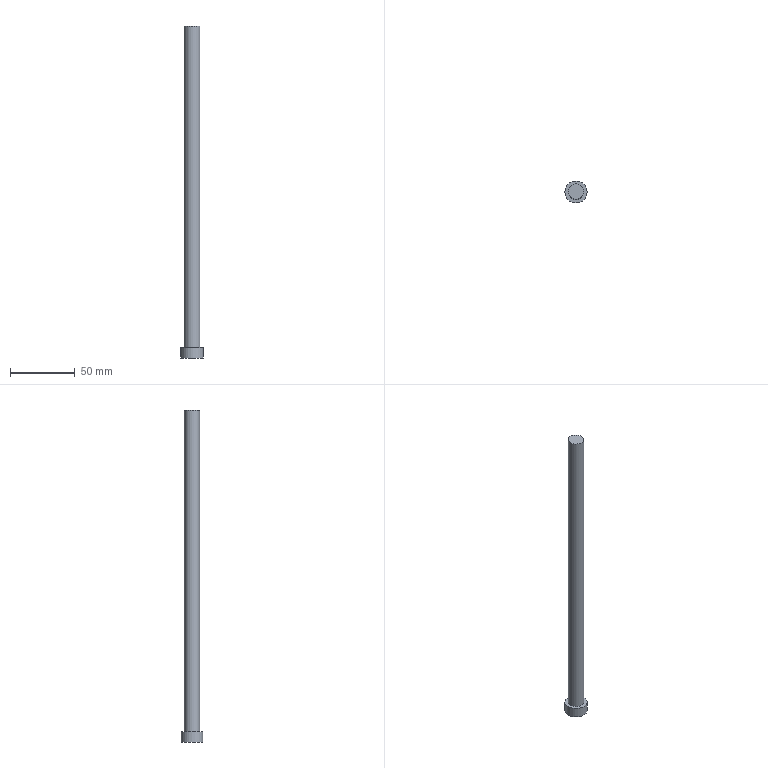Part | NX | features 模具.stp<1>[106] 2 | 1 solid | 5 faces | box 17 x 17 x 255.5 mm | volume 29807 mm3 | plane 3 | cylinder 2 | commonest cylinder face diameters 12 x1 17 x1
STEP:
#1=CARTESIAN_POINT('',(109.,0.,40.));
#2=VERTEX_POINT('',#1);
#3=CARTESIAN_POINT('',(115.,0.,40.));
#4=DIRECTION('',(0.,0.,-1.));
#5=DIRECTION('',(-1.,0.,0.));
#6=AXIS2_PLACEMENT_3D('',#3,#4,#5);
#7=CIRCLE('',#6,6.);
#8=EDGE_CURVE('',#2,#2,#7,.T.);
#9=ORIENTED_EDGE('',*,*,#8,.F.);
#10=EDGE_LOOP('',(#9));
#11=FACE_BOUND('',#10,.T.);
#12=CARTESIAN_POINT('',(0.,0.,40.));
#13=DIRECTION('',(0.,0.,-1.));
#14=DIRECTION('',(0.,-1.,0.));
#15=AXIS2_PLACEMENT_3D('',#12,#13,#14);
#16=PLANE('',#15);
#17=ADVANCED_FACE('',(#11),#16,.F.);
#18=CARTESIAN_POINT('',(123.5,0.,-215.5));
#19=VERTEX_POINT('',#18);
#20=CARTESIAN_POINT('',(115.,0.,-215.5));
#21=DIRECTION('',(0.,0.,1.));
#22=DIRECTION('',(1.,0.,0.));
#23=AXIS2_PLACEMENT_3D('',#20,#21,#22);
#24=CIRCLE('',#23,8.5);
#25=EDGE_CURVE('',#19,#19,#24,.T.);
#26=ORIENTED_EDGE('',*,*,#25,.T.);
#27=EDGE_LOOP('',(#26));
#28=FACE_BOUND('',#27,.T.);
#29=CARTESIAN_POINT('',(123.5,0.,-207.5));
#30=VERTEX_POINT('',#29);
#31=CARTESIAN_POINT('',(115.,0.,-207.5));
#32=DIRECTION('',(0.,0.,-1.));
#33=DIRECTION('',(1.,0.,0.));
#34=AXIS2_PLACEMENT_3D('',#31,#32,#33);
#35=CIRCLE('',#34,8.5);
#36=EDGE_CURVE('',#30,#30,#35,.T.);
#37=ORIENTED_EDGE('',*,*,#36,.T.);
#38=EDGE_LOOP('',(#37));
#39=FACE_BOUND('',#38,.T.);
#40=CARTESIAN_POINT('',(115.,0.,-215.5));
#41=DIRECTION('',(0.,0.,1.));
#42=DIRECTION('',(1.,0.,0.));
#43=AXIS2_PLACEMENT_3D('',#40,#41,#42);
#44=CYLINDRICAL_SURFACE('',#43,8.5);
#45=ADVANCED_FACE('',(#28,#39),#44,.T.);
#46=ORIENTED_EDGE('',*,*,#25,.F.);
#47=EDGE_LOOP('',(#46));
#48=FACE_BOUND('',#47,.T.);
#49=CARTESIAN_POINT('',(115.,0.,-215.5));
#50=DIRECTION('',(0.,0.,-1.));
#51=DIRECTION('',(0.,-1.,0.));
#52=AXIS2_PLACEMENT_3D('',#49,#50,#51);
#53=PLANE('',#52);
#54=ADVANCED_FACE('',(#48),#53,.T.);
#55=ORIENTED_EDGE('',*,*,#36,.F.);
#56=EDGE_LOOP('',(#55));
#57=FACE_BOUND('',#56,.T.);
#58=CARTESIAN_POINT('',(121.,0.,-207.5));
#59=VERTEX_POINT('',#58);
#60=CARTESIAN_POINT('',(115.,0.,-207.5));
#61=DIRECTION('',(0.,0.,1.));
#62=DIRECTION('',(1.,0.,0.));
#63=AXIS2_PLACEMENT_3D('',#60,#61,#62);
#64=CIRCLE('',#63,6.);
#65=EDGE_CURVE('',#59,#59,#64,.T.);
#66=ORIENTED_EDGE('',*,*,#65,.F.);
#67=EDGE_LOOP('',(#66));
#68=FACE_BOUND('',#67,.T.);
#69=CARTESIAN_POINT('',(115.,0.,-207.5));
#70=DIRECTION('',(0.,0.,1.));
#71=DIRECTION('',(1.,0.,0.));
#72=AXIS2_PLACEMENT_3D('',#69,#70,#71);
#73=PLANE('',#72);
#74=ADVANCED_FACE('',(#57,#68),#73,.T.);
#75=ORIENTED_EDGE('',*,*,#8,.T.);
#76=EDGE_LOOP('',(#75));
#77=FACE_BOUND('',#76,.T.);
#78=ORIENTED_EDGE('',*,*,#65,.T.);
#79=EDGE_LOOP('',(#78));
#80=FACE_BOUND('',#79,.T.);
#81=CARTESIAN_POINT('',(115.,0.,-215.5));
#82=DIRECTION('',(0.,0.,1.));
#83=DIRECTION('',(1.,0.,0.));
#84=AXIS2_PLACEMENT_3D('',#81,#82,#83);
#85=CYLINDRICAL_SURFACE('',#84,6.);
#86=ADVANCED_FACE('',(#77,#80),#85,.T.);
#87=CLOSED_SHELL('',(#17,#45,#54,#74,#86));
#88=MANIFOLD_SOLID_BREP('',#87);
#89=(LENGTH_UNIT()NAMED_UNIT(*)SI_UNIT(.MILLI.,.METRE.));
#90=UNCERTAINTY_MEASURE_WITH_UNIT(LENGTH_MEASURE(0.00001),#89,'','');
#91=(NAMED_UNIT(*)PLANE_ANGLE_UNIT()SI_UNIT($,.RADIAN.));
#92=(NAMED_UNIT(*)SI_UNIT($,.STERADIAN.)SOLID_ANGLE_UNIT());
#93=(GEOMETRIC_REPRESENTATION_CONTEXT(3)GLOBAL_UNCERTAINTY_ASSIGNED_CONTEXT((#90))GLOBAL_UNIT_ASSIGNED_CONTEXT((#89,#91,#92))REPRESENTATION_CONTEXT('',''));
#94=ADVANCED_BREP_SHAPE_REPRESENTATION('',(#88),#93);